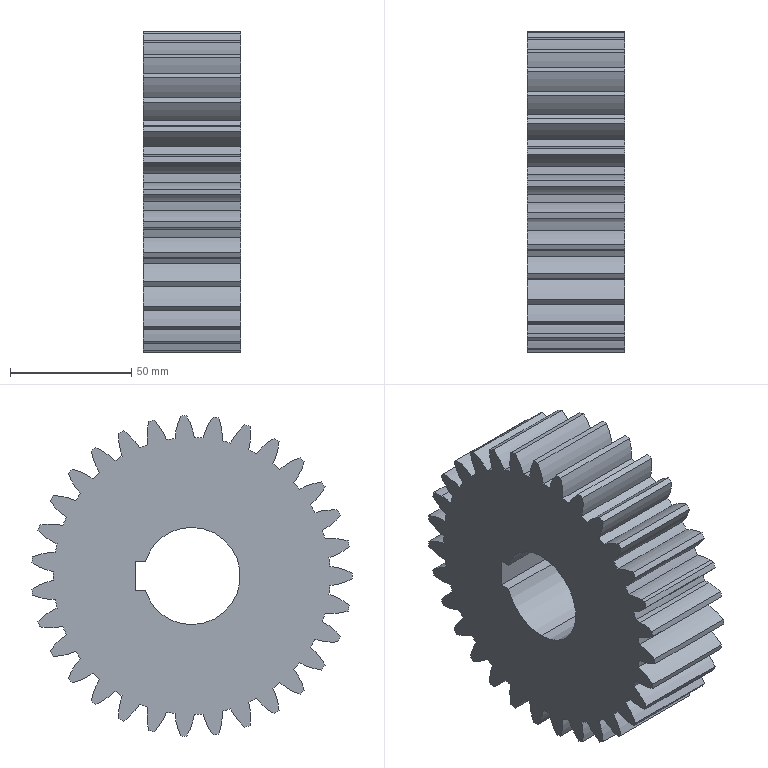Part | SolidWorks | features MBimport 1 | 1 solid | 136 faces | box 40 x 131.774 x 131.932 mm | volume 421323 mm3 | cylinder 131 | plane 5 | commonest cylinder face diameters 49.6 x66 113.998 x31 132 x31 40 x3